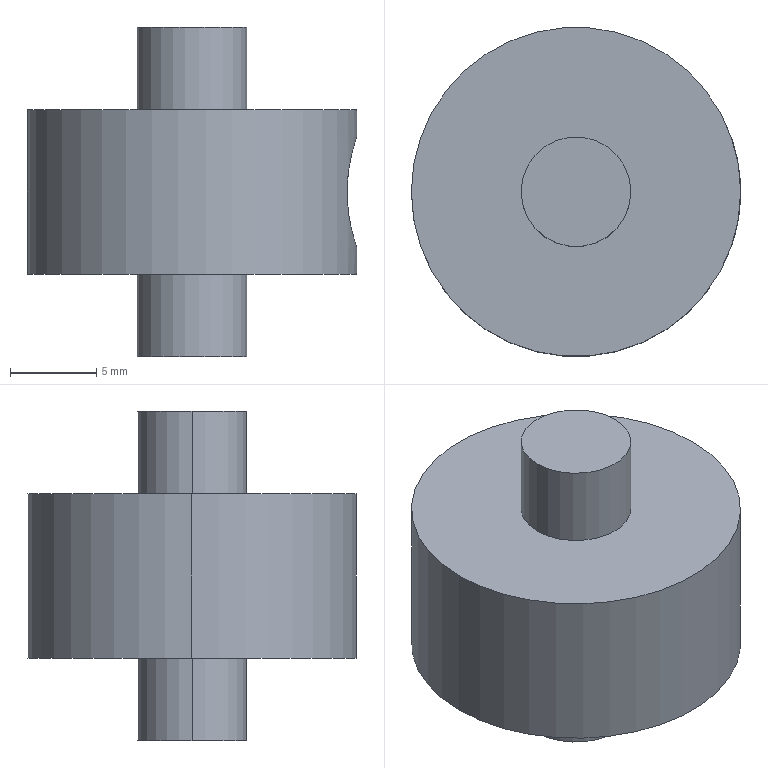Part | SolidWorks | features ICE 3, Extrusion 1 | 1 solid | 13 faces | box 19.05 x 19.05 x 19.05 mm | volume 2719 mm3 | cylinder 8 | plane 5 | commonest cylinder face diameters 6.35 x6 19.05 x2
STEP:
#1=CARTESIAN_POINT('',(9.525,0.,-7.938));
#2=VERTEX_POINT('',#1);
#3=CARTESIAN_POINT('',(9.525,0.,-1.588));
#4=VERTEX_POINT('',#3);
#5=CARTESIAN_POINT('',(9.525,0.,-7.938));
#6=CARTESIAN_POINT('',(9.525,-0.2082,-7.937));
#7=CARTESIAN_POINT('',(9.518,-0.4179,-7.917));
#8=CARTESIAN_POINT('',(9.491,-0.8298,-7.834));
#9=CARTESIAN_POINT('',(9.471,-1.028,-7.774));
#10=CARTESIAN_POINT('',(9.422,-1.411,-7.614));
#11=CARTESIAN_POINT('',(9.392,-1.597,-7.514));
#12=CARTESIAN_POINT('',(9.327,-1.94,-7.284));
#13=CARTESIAN_POINT('',(9.292,-2.099,-7.154));
#14=CARTESIAN_POINT('',(9.185,-2.539,-6.714));
#15=CARTESIAN_POINT('',(9.115,-2.771,-6.368));
#16=CARTESIAN_POINT('',(9.037,-3.012,-5.789));
#17=CARTESIAN_POINT('',(9.016,-3.072,-5.591));
#18=CARTESIAN_POINT('',(8.988,-3.154,-5.183));
#19=CARTESIAN_POINT('',(8.98,-3.175,-4.971));
#20=CARTESIAN_POINT('',(8.98,-3.175,-4.553));
#21=CARTESIAN_POINT('',(8.988,-3.154,-4.346));
#22=CARTESIAN_POINT('',(9.016,-3.073,-3.935));
#23=CARTESIAN_POINT('',(9.037,-3.011,-3.733));
#24=CARTESIAN_POINT('',(9.089,-2.852,-3.351));
#25=CARTESIAN_POINT('',(9.119,-2.753,-3.168));
#26=CARTESIAN_POINT('',(9.186,-2.522,-2.822));
#27=CARTESIAN_POINT('',(9.221,-2.391,-2.663));
#28=CARTESIAN_POINT('',(9.292,-2.1,-2.372));
#29=CARTESIAN_POINT('',(9.327,-1.938,-2.239));
#30=CARTESIAN_POINT('',(9.392,-1.595,-2.009));
#31=CARTESIAN_POINT('',(9.422,-1.413,-1.912));
#32=CARTESIAN_POINT('',(9.471,-1.029,-1.752));
#33=CARTESIAN_POINT('',(9.491,-0.8268,-1.69));
#34=CARTESIAN_POINT('',(9.518,-0.419,-1.608));
#35=CARTESIAN_POINT('',(9.525,-0.2114,-1.588));
#36=CARTESIAN_POINT('',(9.525,0.,-1.588));
#37=B_SPLINE_CURVE_WITH_KNOTS('',3,(#5,#6,#7,#8,#9,#10,#11,#12,#13,#14,#15,#16,#17,#18,#19,#20,#21,#22,#23,#24,#25,#26,#27,#28,#29,#30,#31,#32,#33,#34,#35,#36),.UNSPECIFIED.,.F.,.F.,(4,2,2,2,2,2,2,2,2,2,2,2,2,2,2,4),(0.009999,0.01062,0.01125,0.01187,0.0125,0.01375,0.01437,0.015,0.01562,0.01625,0.01687,0.0175,0.01812,0.01875,0.01937,0.01999),.UNSPECIFIED.);
#38=EDGE_CURVE('',#2,#4,#37,.T.);
#39=ORIENTED_EDGE('',*,*,#38,.F.);
#40=CARTESIAN_POINT('',(0.,0.,-7.938));
#41=VERTEX_POINT('',#40);
#42=CARTESIAN_POINT('',(9.525,0.,-7.938));
#43=DIRECTION('',(-1.,0.,0.));
#44=VECTOR('',#43,1000.);
#45=LINE('',#42,#44);
#46=EDGE_CURVE('',#2,#41,#45,.T.);
#47=ORIENTED_EDGE('',*,*,#46,.T.);
#48=CARTESIAN_POINT('',(0.,0.,-1.587));
#49=VERTEX_POINT('',#48);
#50=CARTESIAN_POINT('',(0.,0.,-4.763));
#51=DIRECTION('',(1.,0.,0.));
#52=DIRECTION('',(0.,0.,-1.));
#53=AXIS2_PLACEMENT_3D('',#50,#51,#52);
#54=CIRCLE('',#53,3.175);
#55=EDGE_CURVE('',#49,#41,#54,.T.);
#56=ORIENTED_EDGE('',*,*,#55,.F.);
#57=CARTESIAN_POINT('',(9.525,0.,-1.587));
#58=DIRECTION('',(-1.,0.,0.));
#59=VECTOR('',#58,1000.);
#60=LINE('',#57,#59);
#61=EDGE_CURVE('',#4,#49,#60,.T.);
#62=ORIENTED_EDGE('',*,*,#61,.F.);
#63=EDGE_LOOP('',(#39,#47,#56,#62));
#64=FACE_OUTER_BOUND('',#63,.T.);
#65=CARTESIAN_POINT('',(9.525,0.,-4.763));
#66=DIRECTION('',(-1.,0.,0.));
#67=DIRECTION('',(0.,0.,1.));
#68=AXIS2_PLACEMENT_3D('',#65,#66,#67);
#69=CYLINDRICAL_SURFACE('',#68,3.175);
#70=ADVANCED_FACE('',(#64),#69,.F.);
#71=CARTESIAN_POINT('',(-3.175,0.,-14.288));
#72=VERTEX_POINT('',#71);
#73=CARTESIAN_POINT('',(3.175,0.,-14.288));
#74=VERTEX_POINT('',#73);
#75=CARTESIAN_POINT('',(0.,0.,-14.288));
#76=DIRECTION('',(0.,0.,-1.));
#77=DIRECTION('',(-1.,0.,0.));
#78=AXIS2_PLACEMENT_3D('',#75,#76,#77);
#79=CIRCLE('',#78,3.175);
#80=EDGE_CURVE('',#72,#74,#79,.T.);
#81=ORIENTED_EDGE('',*,*,#80,.F.);
#82=CARTESIAN_POINT('',(-3.175,0.,-9.525));
#83=VERTEX_POINT('',#82);
#84=CARTESIAN_POINT('',(-3.175,0.,-14.288));
#85=DIRECTION('',(0.,0.,1.));
#86=VECTOR('',#85,1000.);
#87=LINE('',#84,#86);
#88=EDGE_CURVE('',#72,#83,#87,.T.);
#89=ORIENTED_EDGE('',*,*,#88,.T.);
#90=CARTESIAN_POINT('',(3.175,0.,-9.525));
#91=VERTEX_POINT('',#90);
#92=CARTESIAN_POINT('',(0.,0.,-9.525));
#93=DIRECTION('',(0.,0.,-1.));
#94=DIRECTION('',(-1.,0.,0.));
#95=AXIS2_PLACEMENT_3D('',#92,#93,#94);
#96=CIRCLE('',#95,3.175);
#97=EDGE_CURVE('',#83,#91,#96,.T.);
#98=ORIENTED_EDGE('',*,*,#97,.T.);
#99=CARTESIAN_POINT('',(3.175,0.,-14.288));
#100=DIRECTION('',(0.,0.,1.));
#101=VECTOR('',#100,1000.);
#102=LINE('',#99,#101);
#103=EDGE_CURVE('',#74,#91,#102,.T.);
#104=ORIENTED_EDGE('',*,*,#103,.F.);
#105=EDGE_LOOP('',(#81,#89,#98,#104));
#106=FACE_OUTER_BOUND('',#105,.T.);
#107=CARTESIAN_POINT('',(0.,0.,-14.288));
#108=DIRECTION('',(0.,0.,1.));
#109=DIRECTION('',(1.,0.,0.));
#110=AXIS2_PLACEMENT_3D('',#107,#108,#109);
#111=CYLINDRICAL_SURFACE('',#110,3.175);
#112=ADVANCED_FACE('',(#106),#111,.T.);
#113=CARTESIAN_POINT('',(3.175,0.,4.763));
#114=VERTEX_POINT('',#113);
#115=CARTESIAN_POINT('',(-3.175,0.,4.763));
#116=VERTEX_POINT('',#115);
#117=CARTESIAN_POINT('',(0.,0.,4.763));
#118=DIRECTION('',(0.,0.,1.));
#119=DIRECTION('',(1.,0.,0.));
#120=AXIS2_PLACEMENT_3D('',#117,#118,#119);
#121=CIRCLE('',#120,3.175);
#122=EDGE_CURVE('',#114,#116,#121,.T.);
#123=ORIENTED_EDGE('',*,*,#122,.F.);
#124=CARTESIAN_POINT('',(3.175,0.,0.));
#125=VERTEX_POINT('',#124);
#126=CARTESIAN_POINT('',(3.175,0.,4.763));
#127=DIRECTION('',(0.,0.,-1.));
#128=VECTOR('',#127,1000.);
#129=LINE('',#126,#128);
#130=EDGE_CURVE('',#114,#125,#129,.T.);
#131=ORIENTED_EDGE('',*,*,#130,.T.);
#132=CARTESIAN_POINT('',(-3.175,0.,0.));
#133=VERTEX_POINT('',#132);
#134=CARTESIAN_POINT('',(0.,0.,0.));
#135=DIRECTION('',(0.,0.,1.));
#136=DIRECTION('',(1.,0.,0.));
#137=AXIS2_PLACEMENT_3D('',#134,#135,#136);
#138=CIRCLE('',#137,3.175);
#139=EDGE_CURVE('',#125,#133,#138,.T.);
#140=ORIENTED_EDGE('',*,*,#139,.T.);
#141=CARTESIAN_POINT('',(-3.175,0.,4.763));
#142=DIRECTION('',(0.,0.,-1.));
#143=VECTOR('',#142,1000.);
#144=LINE('',#141,#143);
#145=EDGE_CURVE('',#116,#133,#144,.T.);
#146=ORIENTED_EDGE('',*,*,#145,.F.);
#147=EDGE_LOOP('',(#123,#131,#140,#146));
#148=FACE_OUTER_BOUND('',#147,.T.);
#149=CARTESIAN_POINT('',(0.,0.,4.763));
#150=DIRECTION('',(0.,0.,-1.));
#151=DIRECTION('',(-1.,0.,0.));
#152=AXIS2_PLACEMENT_3D('',#149,#150,#151);
#153=CYLINDRICAL_SURFACE('',#152,3.175);
#154=ADVANCED_FACE('',(#148),#153,.T.);
#155=CARTESIAN_POINT('',(9.525,0.,-9.525));
#156=VERTEX_POINT('',#155);
#157=CARTESIAN_POINT('',(-9.525,0.,-9.525));
#158=VERTEX_POINT('',#157);
#159=CARTESIAN_POINT('',(0.,0.,-9.525));
#160=DIRECTION('',(0.,0.,1.));
#161=DIRECTION('',(1.,0.,0.));
#162=AXIS2_PLACEMENT_3D('',#159,#160,#161);
#163=CIRCLE('',#162,9.525);
#164=EDGE_CURVE('',#156,#158,#163,.T.);
#165=ORIENTED_EDGE('',*,*,#164,.T.);
#166=CARTESIAN_POINT('',(-9.525,0.,0.));
#167=VERTEX_POINT('',#166);
#168=CARTESIAN_POINT('',(-9.525,0.,-9.525));
#169=DIRECTION('',(0.,0.,1.));
#170=VECTOR('',#169,1000.);
#171=LINE('',#168,#170);
#172=EDGE_CURVE('',#158,#167,#171,.T.);
#173=ORIENTED_EDGE('',*,*,#172,.T.);
#174=CARTESIAN_POINT('',(9.525,0.,0.));
#175=VERTEX_POINT('',#174);
#176=CARTESIAN_POINT('',(0.,0.,0.));
#177=DIRECTION('',(0.,0.,1.));
#178=DIRECTION('',(1.,0.,0.));
#179=AXIS2_PLACEMENT_3D('',#176,#177,#178);
#180=CIRCLE('',#179,9.525);
#181=EDGE_CURVE('',#175,#167,#180,.T.);
#182=ORIENTED_EDGE('',*,*,#181,.F.);
#183=CARTESIAN_POINT('',(9.525,0.,-9.525));
#184=DIRECTION('',(0.,0.,1.));
#185=VECTOR('',#184,1000.);
#186=LINE('',#183,#185);
#187=EDGE_CURVE('',#4,#175,#186,.T.);
#188=ORIENTED_EDGE('',*,*,#187,.F.);
#189=CARTESIAN_POINT('',(9.525,0.,-1.588));
#190=CARTESIAN_POINT('',(9.525,0.2114,-1.587));
#191=CARTESIAN_POINT('',(9.518,0.419,-1.608));
#192=CARTESIAN_POINT('',(9.491,0.8269,-1.69));
#193=CARTESIAN_POINT('',(9.471,1.029,-1.752));
#194=CARTESIAN_POINT('',(9.422,1.413,-1.912));
#195=CARTESIAN_POINT('',(9.392,1.595,-2.01));
#196=CARTESIAN_POINT('',(9.327,1.939,-2.24));
#197=CARTESIAN_POINT('',(9.292,2.101,-2.373));
#198=CARTESIAN_POINT('',(9.186,2.537,-2.809));
#199=CARTESIAN_POINT('',(9.114,2.772,-3.161));
#200=CARTESIAN_POINT('',(9.037,3.011,-3.733));
#201=CARTESIAN_POINT('',(9.016,3.072,-3.935));
#202=CARTESIAN_POINT('',(8.988,3.154,-4.345));
#203=CARTESIAN_POINT('',(8.98,3.175,-4.552));
#204=CARTESIAN_POINT('',(8.98,3.175,-4.97));
#205=CARTESIAN_POINT('',(8.988,3.154,-5.182));
#206=CARTESIAN_POINT('',(9.016,3.072,-5.59));
#207=CARTESIAN_POINT('',(9.037,3.012,-5.789));
#208=CARTESIAN_POINT('',(9.089,2.851,-6.175));
#209=CARTESIAN_POINT('',(9.119,2.752,-6.358));
#210=CARTESIAN_POINT('',(9.186,2.523,-6.701));
#211=CARTESIAN_POINT('',(9.221,2.39,-6.862));
#212=CARTESIAN_POINT('',(9.292,2.098,-7.154));
#213=CARTESIAN_POINT('',(9.327,1.939,-7.285));
#214=CARTESIAN_POINT('',(9.392,1.596,-7.515));
#215=CARTESIAN_POINT('',(9.422,1.41,-7.615));
#216=CARTESIAN_POINT('',(9.471,1.028,-7.774));
#217=CARTESIAN_POINT('',(9.491,0.8299,-7.834));
#218=CARTESIAN_POINT('',(9.518,0.4188,-7.917));
#219=CARTESIAN_POINT('',(9.525,0.2083,-7.938));
#220=CARTESIAN_POINT('',(9.525,0.,-7.938));
#221=B_SPLINE_CURVE_WITH_KNOTS('',3,(#189,#190,#191,#192,#193,#194,#195,#196,#197,#198,#199,#200,#201,#202,#203,#204,#205,#206,#207,#208,#209,#210,#211,#212,#213,#214,#215,#216,#217,#218,#219,#220),.UNSPECIFIED.,.F.,.F.,(4,2,2,2,2,2,2,2,2,2,2,2,2,2,2,4),(0.,0.0006249,0.00125,0.001875,0.0025,0.003749,0.004374,0.004999,0.005624,0.006249,0.006874,0.007499,0.008124,0.008749,0.009374,0.009999),.UNSPECIFIED.);
#222=EDGE_CURVE('',#4,#2,#221,.T.);
#223=ORIENTED_EDGE('',*,*,#222,.T.);
#224=CARTESIAN_POINT('',(9.525,0.,-9.525));
#225=DIRECTION('',(0.,0.,1.));
#226=VECTOR('',#225,1000.);
#227=LINE('',#224,#226);
#228=EDGE_CURVE('',#156,#2,#227,.T.);
#229=ORIENTED_EDGE('',*,*,#228,.F.);
#230=EDGE_LOOP('',(#165,#173,#182,#188,#223,#229));
#231=FACE_OUTER_BOUND('',#230,.T.);
#232=CARTESIAN_POINT('',(0.,0.,-9.525));
#233=DIRECTION('',(0.,0.,1.));
#234=DIRECTION('',(1.,0.,0.));
#235=AXIS2_PLACEMENT_3D('',#232,#233,#234);
#236=CYLINDRICAL_SURFACE('',#235,9.525);
#237=ADVANCED_FACE('',(#231),#236,.T.);
#238=ORIENTED_EDGE('',*,*,#172,.F.);
#239=CARTESIAN_POINT('',(0.,0.,-9.525));
#240=DIRECTION('',(0.,0.,1.));
#241=DIRECTION('',(1.,0.,0.));
#242=AXIS2_PLACEMENT_3D('',#239,#240,#241);
#243=CIRCLE('',#242,9.525);
#244=EDGE_CURVE('',#158,#156,#243,.T.);
#245=ORIENTED_EDGE('',*,*,#244,.T.);
#246=ORIENTED_EDGE('',*,*,#228,.T.);
#247=ORIENTED_EDGE('',*,*,#38,.T.);
#248=ORIENTED_EDGE('',*,*,#187,.T.);
#249=CARTESIAN_POINT('',(0.,0.,0.));
#250=DIRECTION('',(0.,0.,1.));
#251=DIRECTION('',(1.,0.,0.));
#252=AXIS2_PLACEMENT_3D('',#249,#250,#251);
#253=CIRCLE('',#252,9.525);
#254=EDGE_CURVE('',#167,#175,#253,.T.);
#255=ORIENTED_EDGE('',*,*,#254,.F.);
#256=EDGE_LOOP('',(#238,#245,#246,#247,#248,#255));
#257=FACE_OUTER_BOUND('',#256,.T.);
#258=CARTESIAN_POINT('',(0.,0.,-9.525));
#259=DIRECTION('',(0.,0.,1.));
#260=DIRECTION('',(1.,0.,0.));
#261=AXIS2_PLACEMENT_3D('',#258,#259,#260);
#262=CYLINDRICAL_SURFACE('',#261,9.525);
#263=ADVANCED_FACE('',(#257),#262,.T.);
#264=CARTESIAN_POINT('',(0.,0.,-9.525));
#265=DIRECTION('',(0.,0.,-1.));
#266=DIRECTION('',(-1.,0.,0.));
#267=AXIS2_PLACEMENT_3D('',#264,#265,#266);
#268=CIRCLE('',#267,3.175);
#269=EDGE_CURVE('',#91,#83,#268,.T.);
#270=ORIENTED_EDGE('',*,*,#269,.F.);
#271=ORIENTED_EDGE('',*,*,#97,.F.);
#272=EDGE_LOOP('',(#270,#271));
#273=FACE_BOUND('',#272,.T.);
#274=ORIENTED_EDGE('',*,*,#164,.F.);
#275=ORIENTED_EDGE('',*,*,#244,.F.);
#276=EDGE_LOOP('',(#274,#275));
#277=FACE_OUTER_BOUND('',#276,.T.);
#278=CARTESIAN_POINT('',(0.,0.,-9.525));
#279=DIRECTION('',(0.,0.,1.));
#280=DIRECTION('',(1.,0.,0.));
#281=AXIS2_PLACEMENT_3D('',#278,#279,#280);
#282=PLANE('',#281);
#283=ADVANCED_FACE('',(#273,#277),#282,.F.);
#284=CARTESIAN_POINT('',(0.,0.,0.));
#285=DIRECTION('',(0.,0.,1.));
#286=DIRECTION('',(1.,0.,0.));
#287=AXIS2_PLACEMENT_3D('',#284,#285,#286);
#288=CIRCLE('',#287,3.175);
#289=EDGE_CURVE('',#133,#125,#288,.T.);
#290=ORIENTED_EDGE('',*,*,#289,.F.);
#291=ORIENTED_EDGE('',*,*,#139,.F.);
#292=EDGE_LOOP('',(#290,#291));
#293=FACE_BOUND('',#292,.T.);
#294=ORIENTED_EDGE('',*,*,#181,.T.);
#295=ORIENTED_EDGE('',*,*,#254,.T.);
#296=EDGE_LOOP('',(#294,#295));
#297=FACE_OUTER_BOUND('',#296,.T.);
#298=CARTESIAN_POINT('',(0.,0.,0.));
#299=DIRECTION('',(0.,0.,1.));
#300=DIRECTION('',(1.,0.,0.));
#301=AXIS2_PLACEMENT_3D('',#298,#299,#300);
#302=PLANE('',#301);
#303=ADVANCED_FACE('',(#293,#297),#302,.T.);
#304=ORIENTED_EDGE('',*,*,#130,.F.);
#305=CARTESIAN_POINT('',(0.,0.,4.763));
#306=DIRECTION('',(0.,0.,1.));
#307=DIRECTION('',(1.,0.,0.));
#308=AXIS2_PLACEMENT_3D('',#305,#306,#307);
#309=CIRCLE('',#308,3.175);
#310=EDGE_CURVE('',#116,#114,#309,.T.);
#311=ORIENTED_EDGE('',*,*,#310,.F.);
#312=ORIENTED_EDGE('',*,*,#145,.T.);
#313=ORIENTED_EDGE('',*,*,#289,.T.);
#314=EDGE_LOOP('',(#304,#311,#312,#313));
#315=FACE_OUTER_BOUND('',#314,.T.);
#316=CARTESIAN_POINT('',(0.,0.,4.763));
#317=DIRECTION('',(0.,0.,-1.));
#318=DIRECTION('',(-1.,0.,0.));
#319=AXIS2_PLACEMENT_3D('',#316,#317,#318);
#320=CYLINDRICAL_SURFACE('',#319,3.175);
#321=ADVANCED_FACE('',(#315),#320,.T.);
#322=ORIENTED_EDGE('',*,*,#310,.T.);
#323=ORIENTED_EDGE('',*,*,#122,.T.);
#324=EDGE_LOOP('',(#322,#323));
#325=FACE_OUTER_BOUND('',#324,.T.);
#326=CARTESIAN_POINT('',(0.,0.,4.763));
#327=DIRECTION('',(0.,0.,1.));
#328=DIRECTION('',(1.,0.,0.));
#329=AXIS2_PLACEMENT_3D('',#326,#327,#328);
#330=PLANE('',#329);
#331=ADVANCED_FACE('',(#325),#330,.T.);
#332=ORIENTED_EDGE('',*,*,#88,.F.);
#333=CARTESIAN_POINT('',(0.,0.,-14.288));
#334=DIRECTION('',(0.,0.,-1.));
#335=DIRECTION('',(-1.,0.,0.));
#336=AXIS2_PLACEMENT_3D('',#333,#334,#335);
#337=CIRCLE('',#336,3.175);
#338=EDGE_CURVE('',#74,#72,#337,.T.);
#339=ORIENTED_EDGE('',*,*,#338,.F.);
#340=ORIENTED_EDGE('',*,*,#103,.T.);
#341=ORIENTED_EDGE('',*,*,#269,.T.);
#342=EDGE_LOOP('',(#332,#339,#340,#341));
#343=FACE_OUTER_BOUND('',#342,.T.);
#344=CARTESIAN_POINT('',(0.,0.,-14.288));
#345=DIRECTION('',(0.,0.,1.));
#346=DIRECTION('',(1.,0.,0.));
#347=AXIS2_PLACEMENT_3D('',#344,#345,#346);
#348=CYLINDRICAL_SURFACE('',#347,3.175);
#349=ADVANCED_FACE('',(#343),#348,.T.);
#350=ORIENTED_EDGE('',*,*,#338,.T.);
#351=ORIENTED_EDGE('',*,*,#80,.T.);
#352=EDGE_LOOP('',(#350,#351));
#353=FACE_OUTER_BOUND('',#352,.T.);
#354=CARTESIAN_POINT('',(0.,0.,-14.288));
#355=DIRECTION('',(0.,0.,-1.));
#356=DIRECTION('',(-1.,0.,0.));
#357=AXIS2_PLACEMENT_3D('',#354,#355,#356);
#358=PLANE('',#357);
#359=ADVANCED_FACE('',(#353),#358,.T.);
#360=ORIENTED_EDGE('',*,*,#46,.F.);
#361=ORIENTED_EDGE('',*,*,#222,.F.);
#362=ORIENTED_EDGE('',*,*,#61,.T.);
#363=CARTESIAN_POINT('',(0.,0.,-4.763));
#364=DIRECTION('',(1.,0.,0.));
#365=DIRECTION('',(0.,0.,-1.));
#366=AXIS2_PLACEMENT_3D('',#363,#364,#365);
#367=CIRCLE('',#366,3.175);
#368=EDGE_CURVE('',#41,#49,#367,.T.);
#369=ORIENTED_EDGE('',*,*,#368,.F.);
#370=EDGE_LOOP('',(#360,#361,#362,#369));
#371=FACE_OUTER_BOUND('',#370,.T.);
#372=CARTESIAN_POINT('',(9.525,0.,-4.763));
#373=DIRECTION('',(-1.,0.,0.));
#374=DIRECTION('',(0.,0.,1.));
#375=AXIS2_PLACEMENT_3D('',#372,#373,#374);
#376=CYLINDRICAL_SURFACE('',#375,3.175);
#377=ADVANCED_FACE('',(#371),#376,.F.);
#378=ORIENTED_EDGE('',*,*,#55,.T.);
#379=ORIENTED_EDGE('',*,*,#368,.T.);
#380=EDGE_LOOP('',(#378,#379));
#381=FACE_OUTER_BOUND('',#380,.T.);
#382=CARTESIAN_POINT('',(0.,0.,-4.763));
#383=DIRECTION('',(1.,0.,0.));
#384=DIRECTION('',(0.,0.,-1.));
#385=AXIS2_PLACEMENT_3D('',#382,#383,#384);
#386=PLANE('',#385);
#387=ADVANCED_FACE('',(#381),#386,.T.);
#388=CLOSED_SHELL('',(#70,#112,#154,#237,#263,#283,#303,#321,#331,#349,#359,#377,#387));
#389=MANIFOLD_SOLID_BREP('',#388);
#390=CARTESIAN_POINT('',(0.,0.,0.));
#391=DIRECTION('',(0.,0.,1.));
#392=DIRECTION('',(1.,0.,0.));
#393=AXIS2_PLACEMENT_3D('',#390,#391,#392);
#394=(LENGTH_UNIT()NAMED_UNIT(*)SI_UNIT(.MILLI.,.METRE.));
#395=UNCERTAINTY_MEASURE_WITH_UNIT(LENGTH_MEASURE(0.00001),#394,'','');
#396=(NAMED_UNIT(*)PLANE_ANGLE_UNIT()SI_UNIT($,.RADIAN.));
#397=(NAMED_UNIT(*)SI_UNIT($,.STERADIAN.)SOLID_ANGLE_UNIT());
#398=(GEOMETRIC_REPRESENTATION_CONTEXT(3)GLOBAL_UNCERTAINTY_ASSIGNED_CONTEXT((#395))GLOBAL_UNIT_ASSIGNED_CONTEXT((#394,#396,#397))REPRESENTATION_CONTEXT('',''));
#399=ADVANCED_BREP_SHAPE_REPRESENTATION('',(#389,#393),#398);